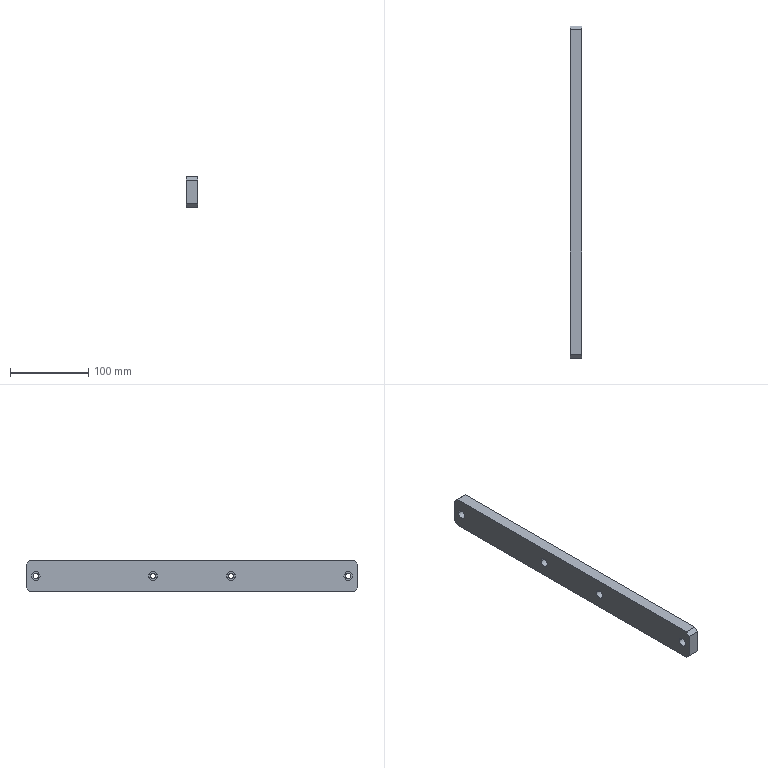Part | STEP file | STOPPER.PAD.stp | 1 solid | 30 faces | box 15 x 425 x 40 mm | volume 250251 mm3 | spline 27 | plane 3